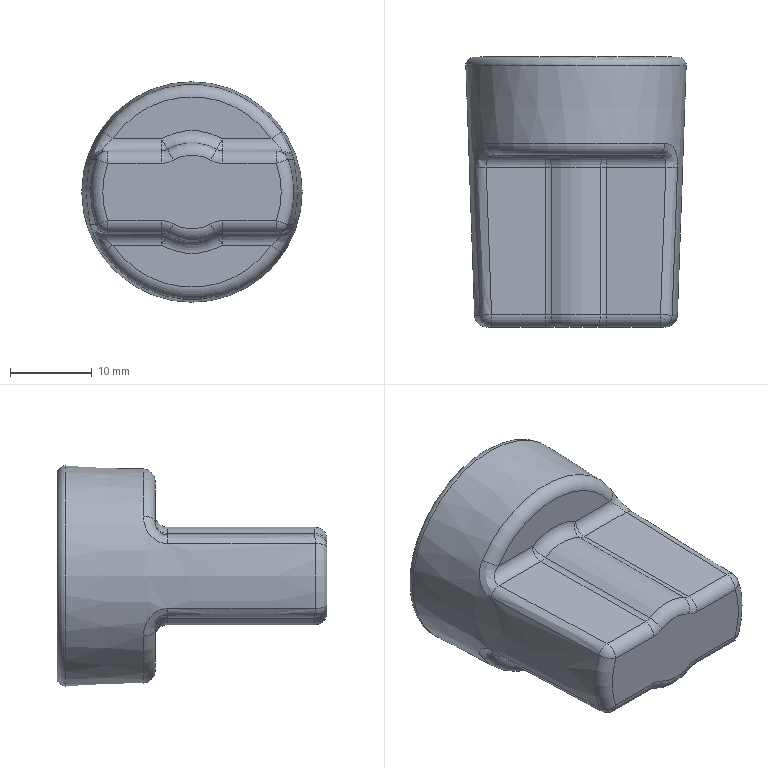Part | STEP file | Lower_shell | 1 solid | 52 faces | box 26.929 x 33 x 26.929 mm | volume 11981 mm3 | cylinder 14 | torus 13 | plane 8 | spline 8 | sphere 8 | cone 1 | commonest cylinder face diameters 3 x12 12 x2